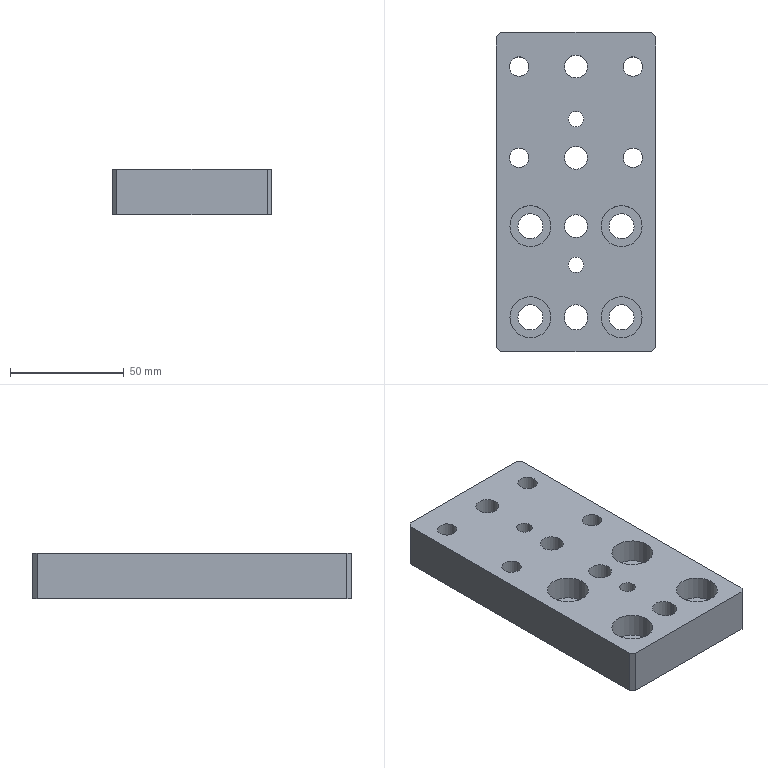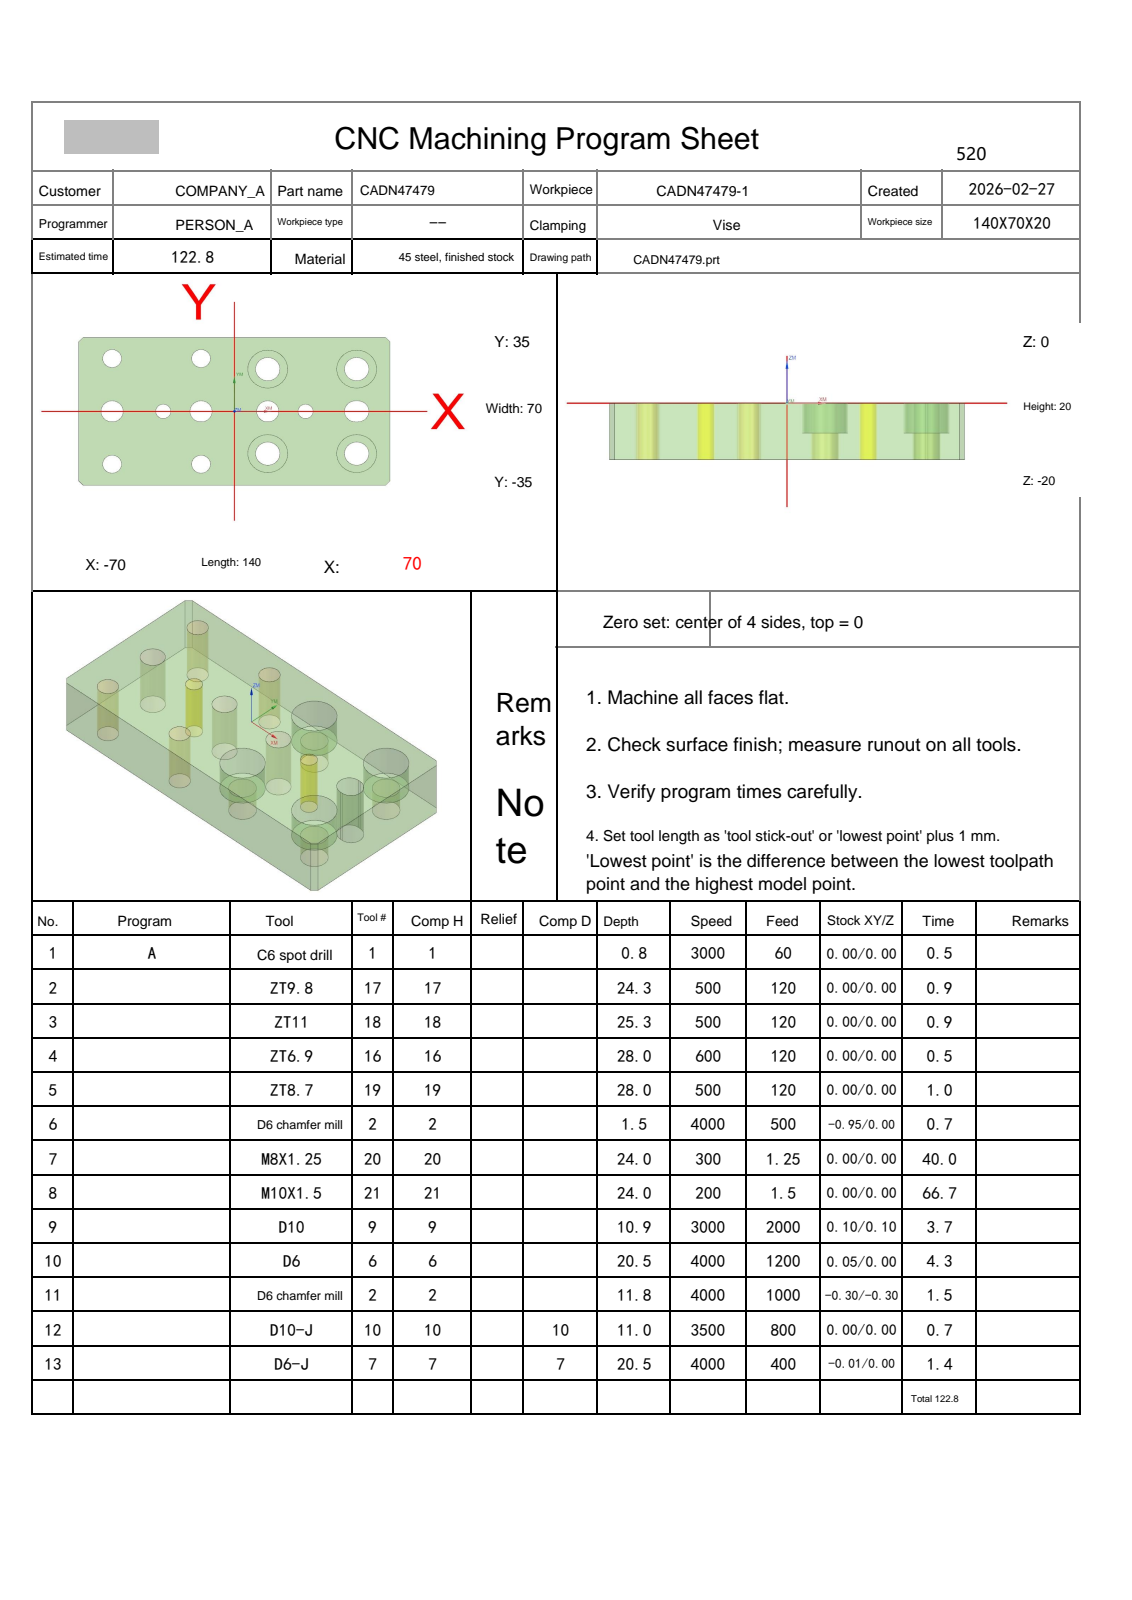NC program | NX | posted by the shop | part box 70 x 140 x 20 mm
Lines 1 to 1647 of 3634, first 1188 of 1645 lines:
%
O0001
(Machine time: 227.62 MIN)
(===Total Tool:12===)
(T1=C6 spot drill   D=6.   R=0.   D-  H01 Z=-0.8  )
(T17=ZT9.8  D=9.8  DR_a=120 D-  H17 Z=-24.33)
(T18=ZT11   D=11.  DR_a=118 D-  H18 Z=-25.3 )
(T16=ZT6.9  D=6.9  DR_a=120 D-  H16 Z=-28.  )
(T19=ZT8.7  D=8.7  DR_a=118 D-  H19 Z=-28.  )
(T2=D6 chamfer mill   D=6.   R=0.   D-  H02 Z=-11.8 )
(T20=M8X1.25 D=6.8  DR_a=180 D-  H20 Z=-24.  )
(T21=M10X1.5 D=8.5  DR_a=180 D-  H21 Z=-24.  )
(T9=D10     D=10.  R=0.   D-  H09 Z=-10.9 )
(T6=D6      D=6.   R=0.   D-  H06 Z=-20.5 )
(T10=D10-J  D=10.  R=0.   D10 H10 Z=-11.  )
(T7=D6-J    D=6.   R=0.   D7  H07 Z=-20.5 )
G80 G90 G17 G49 G40
G91 G28 Z0
M01
N1 T01 M06
(C6 spot drill  D=6. R=0. H=01 ce=0.00 di=0.00)
G00 G90 G54 X55. Y20. M03 S3000
G43 H01 Z30.
M08
G98 G81 X55. Y20. Z-.8 R1. F60.
Y-20.
X32. Y0.0
X15. Y-20.
Y0.0
Y20.
X-15. Y25.
Y0.0
X-32.
X-15. Y-25.
X-55.
Y0.0
Y25.
G80
G00 Z30.
G00 G90 X54.5 Y0.0 M03 S3000
Z30.
G98 G81 X54.5 Y0.0 Z-.8 R1. F60.
G80
G00 Z30.
G91 G28 Z0.0
M05
M09
G91 G28 Z0.0
M01
N2 T17 M06
(ZT9.8 D=9.8 DR_a=120 H=17)
G00 G90 G54 X-55. Y0.0 M03 S500
G43 H17 Z30.
M08
G98 G83 X-55. Y0.0 Z-24.329 R1. F120. Q2.
X-15.
X15.
G80
G00 Z30.
G00 G90 X54.5 Y0.0 M03 S500
Z30.
G98 G83 X54.5 Y0.0 Z-24.329 R1. F120. Q2.
G80
G00 Z30.
G91 G28 Z0.0
M05
M09
G91 G28 Z0.0
M01
N3 T18 M06
(ZT11 D=11. DR_a=118 H=18)
G00 G90 G54 X15. Y-20. M03 S500
G43 H18 Z30.
M08
G98 G83 X15. Y-20. Z-25.305 R1. F120. Q2.
Y20.
X55.
Y-20.
G80
G00 Z30.
G91 G28 Z0.0
M05
M09
G91 G28 Z0.0
M01
N4 T16 M06
(ZT6.9 D=6.9 DR_a=120 H=16)
G00 G90 G54 X-32. Y0.0 M03 S600
G43 H16 Z30.
M08
G98 G83 X-32. Y0.0 Z-28. R1. F120. Q2.
X32.
G80
G00 Z30.
G91 G28 Z0.0
M05
M09
G91 G28 Z0.0
M01
N5 T19 M06
(ZT8.7 D=8.7 DR_a=118 H=19)
G00 G90 G54 X-55. Y-25. M03 S500
G43 H19 Z30.
M08
G98 G83 X-55. Y-25. Z-28. R1. F120. Q2.
X-15.
Y25.
X-55.
G80
G00 Z30.
G91 G28 Z0.0
M05
M09
G91 G28 Z0.0
M01
N6 T02 M06
(D6 chamfer mill  D=6. R=0. H=02 ce=-0.80 di=0.00)
G00 G90 G54 X-33.5 Y-.8 M03 S4000
G43 H02 Z30.
M08
Z-1.
G01 Z-1.5 F500.
Y-1.2
G03 X-32. Y-2.7 I1.5 J0.0
X-29.3 Y0.0 I0.0 J2.7
X-32. Y2.7 I-2.7 J0.0
X-34.7 Y0.0 I0.0 J-2.7
X-32. Y-2.7 I2.7 J0.0
X-30.5 Y-1.2 I0.0 J1.5
G01 Y-.8
Z-1.
G00 Z30.
X30.5
Z-1.
G01 Z-1.5
Y-1.2
G03 X32. Y-2.7 I1.5 J0.0
X34.7 Y0.0 I0.0 J2.7
X32. Y2.7 I-2.7 J0.0
X29.3 Y0.0 I0.0 J-2.7
X32. Y-2.7 I2.7 J0.0
X33.5 Y-1.2 I0.0 J1.5
G01 Y-.8
Z-1.
G00 Z30.
G00 G90 X-57.629 Y24.386 M03 S4000
Z30.
Z-1.
G01 Z-1.5 F500.
X-58. Y24.3
G03 X-55. Y21.3 I3. J0.0
X-51.3 Y25. I0.0 J3.7
X-55. Y28.7 I-3.7 J0.0
X-58.7 Y25. I0.0 J-3.7
X-55. Y21.3 I3.7 J0.0
X-52. Y24.3 I0.0 J3.
G01 X-52.371 Y24.386
Z-1.
G00 Z30.
X-17.629
Z-1.
G01 Z-1.5
X-18. Y24.3
G03 X-15. Y21.3 I3. J0.0
X-11.3 Y25. I0.0 J3.7
X-15. Y28.7 I-3.7 J0.0
X-18.7 Y25. I0.0 J-3.7
X-15. Y21.3 I3.7 J0.0
X-12. Y24.3 I0.0 J3.
G01 X-12.371 Y24.386
Z-1.
G00 Z30.
X-17.629 Y-25.614
Z-1.
G01 Z-1.5
X-18. Y-25.7
G03 X-15. Y-28.7 I3. J0.0
X-11.3 Y-25. I0.0 J3.7
X-15. Y-21.3 I-3.7 J0.0
X-18.7 Y-25. I0.0 J-3.7
X-15. Y-28.7 I3.7 J0.0
X-12. Y-25.7 I0.0 J3.
G01 X-12.371 Y-25.614
Z-1.
G00 Z30.
X-57.629
Z-1.
G01 Z-1.5
X-58. Y-25.7
G03 X-55. Y-28.7 I3. J0.0
X-51.3 Y-25. I0.0 J3.7
X-55. Y-21.3 I-3.7 J0.0
X-58.7 Y-25. I0.0 J-3.7
X-55. Y-28.7 I3.7 J0.0
X-52. Y-25.7 I0.0 J3.
G01 X-52.371 Y-25.614
Z-1.
G00 Z30.
G00 G90 X-58. Y-1.3 M03 S4000
Z30.
Z-.5
G01 Z-1. F500.
G03 X-55. Y-4.3 I3. J0.0
X-50.7 Y0.0 I0.0 J4.3
X-55. Y4.3 I-4.3 J0.0
X-59.3 Y0.0 I0.0 J-4.3
X-55. Y-4.3 I4.3 J0.0
X-52. Y-1.3 I0.0 J3.
G01 Z-.5
G00 Z30.
X-18.
Z-.5
G01 Z-1.
G03 X-15. Y-4.3 I3. J0.0
X-10.7 Y0.0 I0.0 J4.3
X-15. Y4.3 I-4.3 J0.0
X-19.3 Y0.0 I0.0 J-4.3
X-15. Y-4.3 I4.3 J0.0
X-12. Y-1.3 I0.0 J3.
G01 Z-.5
G00 Z30.
X12.
Z-.5
G01 Z-1.
G03 X15. Y-4.3 I3. J0.0
X19.3 Y0.0 I0.0 J4.3
X15. Y4.3 I-4.3 J0.0
X10.7 Y0.0 I0.0 J-4.3
X15. Y-4.3 I4.3 J0.0
X18. Y-1.3 I0.0 J3.
G01 Z-.5
G00 Z30.
G91 G28 Z0.0
M05
M09
G91 G28 Z0.0
M01
N7 T20 M06
(M8X1.25 D=6.8 DR_a=180 H=20)
G00 G90 G54 X-32. Y0.0 M03 S300
G43 H20 Z30.
M08
G95
G98 G84 X-32. Y0.0 Z-24. R1. F1.25 Q3.
X32.
G80
G94
G00 Z30.
G91 G28 Z0.0
M05
M09
G91 G28 Z0.0
M01
N8 T21 M06
(M10X1.5 D=8.5 DR_a=180 H=21)
G00 G90 G54 X-55. Y-25. M03 S200
G43 H21 Z30.
M08
G95
G98 G84 X-55. Y-25. Z-24. R1. F1.5 Q2.
X-15.
Y25.
X-55.
G80
G94
G00 Z30.
G91 G28 Z0.0
M05
M09
G91 G28 Z0.0
M01
N9 T09 M06
(D10  D=10. R=0. H=09 ce=0.10 di=0.10)
G00 G90 G54 X55.636 Y-16.134 M03 S3000
G43 H09 Z30.
M08
Z1.
G01 X54.515 Y-16.1 Z.941 F2000.
X53.275 Y-16.469 Z.873
X52.221 Y-17.221 Z.805
X51.469 Y-18.275 Z.738
X51.1 Y-19.515 Z.67
Y-20.485 Z.619
X51.469 Y-21.725 Z.551
X52.221 Y-22.779 Z.483
X53.275 Y-23.531 Z.415
X54.515 Y-23.9 Z.348
X55.485 Z.297
X56.725 Y-23.531 Z.229
X57.779 Y-22.779 Z.161
X58.531 Y-21.725 Z.093
X58.9 Y-20.485 Z.025
Y-20. Z0.0
G03 X57.321 Y-16.866 Z-.029 I-3.9 J0.0
X55. Y-16.1 Z-.05 I-2.321 J-3.134
X51.1 Y-20. Z-.099 I0.0 J-3.9
X55. Y-23.9 Z-.149 I3.9 J0.0
X58.9 Y-20. Z-.198 I0.0 J3.9
X57.321 Y-16.866 Z-.228 I-3.9 J0.0
X55. Y-16.1 Z-.248 I-2.321 J-3.134
X51.1 Y-20. Z-.297 I0.0 J-3.9
X55. Y-23.9 Z-.347 I3.9 J0.0
X58.9 Y-20. Z-.396 I0.0 J3.9
X57.321 Y-16.866 Z-.426 I-3.9 J0.0
X55. Y-16.1 Z-.446 I-2.321 J-3.134
X51.1 Y-20. Z-.495 I0.0 J-3.9
X55. Y-23.9 Z-.545 I3.9 J0.0
X58.9 Y-20. Z-.594 I0.0 J3.9
X57.321 Y-16.866 Z-.624 I-3.9 J0.0
X55. Y-16.1 Z-.644 I-2.321 J-3.134
X51.1 Y-20. Z-.693 I0.0 J-3.9
X55. Y-23.9 Z-.743 I3.9 J0.0
X58.9 Y-20. Z-.792 I0.0 J3.9
X57.321 Y-16.866 Z-.822 I-3.9 J0.0
X55. Y-16.1 Z-.842 I-2.321 J-3.134
X51.1 Y-20. Z-.892 I0.0 J-3.9
X55. Y-23.9 Z-.941 I3.9 J0.0
X58.9 Y-20. Z-.991 I0.0 J3.9
X57.321 Y-16.866 Z-1.02 I-3.9 J0.0
X55. Y-16.1 Z-1.04 I-2.321 J-3.134
X51.1 Y-20. Z-1.09 I0.0 J-3.9
X55. Y-23.9 Z-1.139 I3.9 J0.0
X58.9 Y-20. Z-1.189 I0.0 J3.9
X57.321 Y-16.866 Z-1.218 I-3.9 J0.0
X55. Y-16.1 Z-1.238 I-2.321 J-3.134
X51.1 Y-20. Z-1.288 I0.0 J-3.9
X55. Y-23.9 Z-1.337 I3.9 J0.0
X58.9 Y-20. Z-1.387 I0.0 J3.9
X57.321 Y-16.866 Z-1.416 I-3.9 J0.0
X55. Y-16.1 Z-1.436 I-2.321 J-3.134
X51.1 Y-20. Z-1.486 I0.0 J-3.9
X55. Y-23.9 Z-1.535 I3.9 J0.0
X58.9 Y-20. Z-1.585 I0.0 J3.9
X57.321 Y-16.866 Z-1.614 I-3.9 J0.0
X55. Y-16.1 Z-1.634 I-2.321 J-3.134
X51.1 Y-20. Z-1.684 I0.0 J-3.9
X55. Y-23.9 Z-1.733 I3.9 J0.0
X58.9 Y-20. Z-1.783 I0.0 J3.9
X57.321 Y-16.866 Z-1.812 I-3.9 J0.0
X55. Y-16.1 Z-1.833 I-2.321 J-3.134
X51.1 Y-20. Z-1.882 I0.0 J-3.9
X55. Y-23.9 Z-1.932 I3.9 J0.0
X58.9 Y-20. Z-1.981 I0.0 J3.9
X57.321 Y-16.866 Z-2.011 I-3.9 J0.0
X55. Y-16.1 Z-2.031 I-2.321 J-3.134
X51.1 Y-20. Z-2.08 I0.0 J-3.9
X55. Y-23.9 Z-2.13 I3.9 J0.0
X58.9 Y-20. Z-2.179 I0.0 J3.9
X57.321 Y-16.866 Z-2.209 I-3.9 J0.0
X55. Y-16.1 Z-2.229 I-2.321 J-3.134
X51.1 Y-20. Z-2.278 I0.0 J-3.9
X55. Y-23.9 Z-2.328 I3.9 J0.0
X58.9 Y-20. Z-2.377 I0.0 J3.9
X57.321 Y-16.866 Z-2.407 I-3.9 J0.0
X55. Y-16.1 Z-2.427 I-2.321 J-3.134
X51.1 Y-20. Z-2.476 I0.0 J-3.9
X55. Y-23.9 Z-2.526 I3.9 J0.0
X58.9 Y-20. Z-2.575 I0.0 J3.9
X57.321 Y-16.866 Z-2.605 I-3.9 J0.0
X55. Y-16.1 Z-2.625 I-2.321 J-3.134
X51.1 Y-20. Z-2.675 I0.0 J-3.9
X55. Y-23.9 Z-2.724 I3.9 J0.0
X58.9 Y-20. Z-2.774 I0.0 J3.9
X57.321 Y-16.866 Z-2.803 I-3.9 J0.0
X55. Y-16.1 Z-2.823 I-2.321 J-3.134
X51.1 Y-20. Z-2.873 I0.0 J-3.9
X55. Y-23.9 Z-2.922 I3.9 J0.0
X58.9 Y-20. Z-2.972 I0.0 J3.9
X57.321 Y-16.866 Z-3.001 I-3.9 J0.0
X55. Y-16.1 Z-3.021 I-2.321 J-3.134
X51.1 Y-20. Z-3.071 I0.0 J-3.9
X55. Y-23.9 Z-3.12 I3.9 J0.0
X58.9 Y-20. Z-3.17 I0.0 J3.9
X57.321 Y-16.866 Z-3.199 I-3.9 J0.0
X55. Y-16.1 Z-3.219 I-2.321 J-3.134
X51.1 Y-20. Z-3.269 I0.0 J-3.9
X55. Y-23.9 Z-3.318 I3.9 J0.0
X58.9 Y-20. Z-3.368 I0.0 J3.9
X57.321 Y-16.866 Z-3.397 I-3.9 J0.0
X55. Y-16.1 Z-3.417 I-2.321 J-3.134
X51.1 Y-20. Z-3.467 I0.0 J-3.9
X55. Y-23.9 Z-3.517 I3.9 J0.0
X58.9 Y-20. Z-3.566 I0.0 J3.9
X57.321 Y-16.866 Z-3.595 I-3.9 J0.0
X55. Y-16.1 Z-3.616 I-2.321 J-3.134
X51.1 Y-20. Z-3.665 I0.0 J-3.9
X55. Y-23.9 Z-3.715 I3.9 J0.0
X58.9 Y-20. Z-3.764 I0.0 J3.9
X57.321 Y-16.866 Z-3.794 I-3.9 J0.0
X55. Y-16.1 Z-3.814 I-2.321 J-3.134
X51.1 Y-20. Z-3.863 I0.0 J-3.9
X55. Y-23.9 Z-3.913 I3.9 J0.0
X58.9 Y-20. Z-3.962 I0.0 J3.9
X57.321 Y-16.866 Z-3.992 I-3.9 J0.0
X55. Y-16.1 Z-4.012 I-2.321 J-3.134
X51.1 Y-20. Z-4.061 I0.0 J-3.9
X55. Y-23.9 Z-4.111 I3.9 J0.0
X58.9 Y-20. Z-4.16 I0.0 J3.9
X57.321 Y-16.866 Z-4.19 I-3.9 J0.0
X55. Y-16.1 Z-4.21 I-2.321 J-3.134
X51.1 Y-20. Z-4.259 I0.0 J-3.9
X55. Y-23.9 Z-4.309 I3.9 J0.0
X58.9 Y-20. Z-4.358 I0.0 J3.9
X57.321 Y-16.866 Z-4.388 I-3.9 J0.0
X55. Y-16.1 Z-4.408 I-2.321 J-3.134
X51.1 Y-20. Z-4.458 I0.0 J-3.9
X55. Y-23.9 Z-4.507 I3.9 J0.0
X58.9 Y-20. Z-4.557 I0.0 J3.9
X57.321 Y-16.866 Z-4.586 I-3.9 J0.0
X55. Y-16.1 Z-4.606 I-2.321 J-3.134
X51.1 Y-20. Z-4.656 I0.0 J-3.9
X55. Y-23.9 Z-4.705 I3.9 J0.0
X58.9 Y-20. Z-4.755 I0.0 J3.9
X57.321 Y-16.866 Z-4.784 I-3.9 J0.0
X55. Y-16.1 Z-4.804 I-2.321 J-3.134
X51.1 Y-20. Z-4.854 I0.0 J-3.9
X55. Y-23.9 Z-4.903 I3.9 J0.0
X58.9 Y-20. Z-4.953 I0.0 J3.9
X57.321 Y-16.866 Z-4.982 I-3.9 J0.0
X55. Y-16.1 Z-5.002 I-2.321 J-3.134
X51.1 Y-20. Z-5.052 I0.0 J-3.9
X55. Y-23.9 Z-5.101 I3.9 J0.0
X58.9 Y-20. Z-5.151 I0.0 J3.9
X57.321 Y-16.866 Z-5.18 I-3.9 J0.0
X55. Y-16.1 Z-5.2 I-2.321 J-3.134
X51.1 Y-20. Z-5.25 I0.0 J-3.9
X55. Y-23.9 Z-5.3 I3.9 J0.0
X58.9 Y-20. Z-5.349 I0.0 J3.9
X57.321 Y-16.866 Z-5.378 I-3.9 J0.0
X55. Y-16.1 Z-5.399 I-2.321 J-3.134
X51.1 Y-20. Z-5.448 I0.0 J-3.9
X55. Y-23.9 Z-5.498 I3.9 J0.0
X58.9 Y-20. Z-5.547 I0.0 J3.9
X57.321 Y-16.866 Z-5.577 I-3.9 J0.0
X55. Y-16.1 Z-5.597 I-2.321 J-3.134
X51.1 Y-20. Z-5.646 I0.0 J-3.9
X55. Y-23.9 Z-5.696 I3.9 J0.0
X58.9 Y-20. Z-5.745 I0.0 J3.9
X57.321 Y-16.866 Z-5.775 I-3.9 J0.0
X55. Y-16.1 Z-5.795 I-2.321 J-3.134
X51.1 Y-20. Z-5.844 I0.0 J-3.9
X55. Y-23.9 Z-5.894 I3.9 J0.0
X58.9 Y-20. Z-5.943 I0.0 J3.9
X57.321 Y-16.866 Z-5.973 I-3.9 J0.0
X55. Y-16.1 Z-5.993 I-2.321 J-3.134
X51.1 Y-20. Z-6.042 I0.0 J-3.9
X55. Y-23.9 Z-6.092 I3.9 J0.0
X58.9 Y-20. Z-6.142 I0.0 J3.9
X57.321 Y-16.866 Z-6.171 I-3.9 J0.0
X55. Y-16.1 Z-6.191 I-2.321 J-3.134
X51.1 Y-20. Z-6.241 I0.0 J-3.9
X55. Y-23.9 Z-6.29 I3.9 J0.0
X58.9 Y-20. Z-6.34 I0.0 J3.9
X57.321 Y-16.866 Z-6.369 I-3.9 J0.0
X55. Y-16.1 Z-6.389 I-2.321 J-3.134
X51.1 Y-20. Z-6.439 I0.0 J-3.9
X55. Y-23.9 Z-6.488 I3.9 J0.0
X58.9 Y-20. Z-6.538 I0.0 J3.9
X57.321 Y-16.866 Z-6.567 I-3.9 J0.0
X55. Y-16.1 Z-6.587 I-2.321 J-3.134
X51.1 Y-20. Z-6.637 I0.0 J-3.9
X55. Y-23.9 Z-6.686 I3.9 J0.0
X58.9 Y-20. Z-6.736 I0.0 J3.9
X57.321 Y-16.866 Z-6.765 I-3.9 J0.0
X55. Y-16.1 Z-6.785 I-2.321 J-3.134
X51.1 Y-20. Z-6.835 I0.0 J-3.9
X55. Y-23.9 Z-6.884 I3.9 J0.0
X58.9 Y-20. Z-6.934 I0.0 J3.9
X57.321 Y-16.866 Z-6.963 I-3.9 J0.0
X55. Y-16.1 Z-6.983 I-2.321 J-3.134
X51.1 Y-20. Z-7.033 I0.0 J-3.9
X55. Y-23.9 Z-7.083 I3.9 J0.0
X58.9 Y-20. Z-7.132 I0.0 J3.9
X57.321 Y-16.866 Z-7.162 I-3.9 J0.0
X55. Y-16.1 Z-7.182 I-2.321 J-3.134
X51.1 Y-20. Z-7.231 I0.0 J-3.9
X55. Y-23.9 Z-7.281 I3.9 J0.0
X58.9 Y-20. Z-7.33 I0.0 J3.9
X57.321 Y-16.866 Z-7.36 I-3.9 J0.0
X55. Y-16.1 Z-7.38 I-2.321 J-3.134
X51.1 Y-20. Z-7.429 I0.0 J-3.9
X55. Y-23.9 Z-7.479 I3.9 J0.0
X58.9 Y-20. Z-7.528 I0.0 J3.9
X57.321 Y-16.866 Z-7.558 I-3.9 J0.0
X55. Y-16.1 Z-7.578 I-2.321 J-3.134
X51.1 Y-20. Z-7.627 I0.0 J-3.9
X55. Y-23.9 Z-7.677 I3.9 J0.0
X58.9 Y-20. Z-7.726 I0.0 J3.9
X57.321 Y-16.866 Z-7.756 I-3.9 J0.0
X55. Y-16.1 Z-7.776 I-2.321 J-3.134
X51.1 Y-20. Z-7.825 I0.0 J-3.9
X55. Y-23.9 Z-7.875 I3.9 J0.0
X58.9 Y-20. Z-7.925 I0.0 J3.9
X57.321 Y-16.866 Z-7.954 I-3.9 J0.0
X55. Y-16.1 Z-7.974 I-2.321 J-3.134
X51.1 Y-20. Z-8.024 I0.0 J-3.9
X55. Y-23.9 Z-8.073 I3.9 J0.0
X58.9 Y-20. Z-8.123 I0.0 J3.9
X57.321 Y-16.866 Z-8.152 I-3.9 J0.0
X55. Y-16.1 Z-8.172 I-2.321 J-3.134
X51.1 Y-20. Z-8.222 I0.0 J-3.9
X55. Y-23.9 Z-8.271 I3.9 J0.0
X58.9 Y-20. Z-8.321 I0.0 J3.9
X57.321 Y-16.866 Z-8.35 I-3.9 J0.0
X55. Y-16.1 Z-8.37 I-2.321 J-3.134
X51.1 Y-20. Z-8.42 I0.0 J-3.9
X55. Y-23.9 Z-8.469 I3.9 J0.0
X58.9 Y-20. Z-8.519 I0.0 J3.9
X57.321 Y-16.866 Z-8.548 I-3.9 J0.0
X55. Y-16.1 Z-8.568 I-2.321 J-3.134
X51.1 Y-20. Z-8.618 I0.0 J-3.9
X55. Y-23.9 Z-8.667 I3.9 J0.0
X58.9 Y-20. Z-8.717 I0.0 J3.9
X57.321 Y-16.866 Z-8.746 I-3.9 J0.0
X55. Y-16.1 Z-8.767 I-2.321 J-3.134
X51.1 Y-20. Z-8.816 I0.0 J-3.9
X55. Y-23.9 Z-8.866 I3.9 J0.0
X58.9 Y-20. Z-8.915 I0.0 J3.9
X57.321 Y-16.866 Z-8.945 I-3.9 J0.0
X55. Y-16.1 Z-8.965 I-2.321 J-3.134
X51.1 Y-20. Z-9.014 I0.0 J-3.9
X55. Y-23.9 Z-9.064 I3.9 J0.0
X58.9 Y-20. Z-9.113 I0.0 J3.9
X57.321 Y-16.866 Z-9.143 I-3.9 J0.0
X55. Y-16.1 Z-9.163 I-2.321 J-3.134
X51.1 Y-20. Z-9.212 I0.0 J-3.9
X55. Y-23.9 Z-9.262 I3.9 J0.0
X58.9 Y-20. Z-9.311 I0.0 J3.9
X57.321 Y-16.866 Z-9.341 I-3.9 J0.0
X55. Y-16.1 Z-9.361 I-2.321 J-3.134
X51.1 Y-20. Z-9.41 I0.0 J-3.9
X55. Y-23.9 Z-9.46 I3.9 J0.0
X58.9 Y-20. Z-9.509 I0.0 J3.9
X57.321 Y-16.866 Z-9.539 I-3.9 J0.0
X55. Y-16.1 Z-9.559 I-2.321 J-3.134
X51.1 Y-20. Z-9.608 I0.0 J-3.9
X55. Y-23.9 Z-9.658 I3.9 J0.0
X58.9 Y-20. Z-9.708 I0.0 J3.9
X57.321 Y-16.866 Z-9.737 I-3.9 J0.0
X55. Y-16.1 Z-9.757 I-2.321 J-3.134
X51.1 Y-20. Z-9.807 I0.0 J-3.9
X55. Y-23.9 Z-9.856 I3.9 J0.0
X58.9 Y-20. Z-9.906 I0.0 J3.9
X57.321 Y-16.866 Z-9.935 I-3.9 J0.0
X55. Y-16.1 Z-9.955 I-2.321 J-3.134
X51.1 Y-20. Z-10.005 I0.0 J-3.9
X55. Y-23.9 Z-10.054 I3.9 J0.0
X58.9 Y-20. Z-10.104 I0.0 J3.9
X57.321 Y-16.866 Z-10.133 I-3.9 J0.0
X55. Y-16.1 Z-10.153 I-2.321 J-3.134
X51.1 Y-20. Z-10.203 I0.0 J-3.9
X55. Y-23.9 Z-10.252 I3.9 J0.0
X58.9 Y-20. Z-10.302 I0.0 J3.9
X57.321 Y-16.866 Z-10.331 I-3.9 J0.0
X55. Y-16.1 Z-10.351 I-2.321 J-3.134
X51.1 Y-20. Z-10.401 I0.0 J-3.9
X55. Y-23.9 Z-10.45 I3.9 J0.0
X58.9 Y-20. Z-10.5 I0.0 J3.9
X55. Y-16.1 I-3.9 J0.0
X51.1 Y-20. I0.0 J-3.9
X55. Y-23.9 I3.9 J0.0
X58.9 Y-20. I0.0 J3.9
X58.88 Y-19.601 I-3.9 J0.0
G01 Z-9.5
G00 Z30.
X18.856 Y-20.634
Z1.
G01 X18.9 Y-20.485 Z.992
Y-19.515 Z.941
X18.531 Y-18.275 Z.873
X17.779 Y-17.221 Z.805
X16.725 Y-16.469 Z.738
X15.485 Y-16.1 Z.67
X14.515 Z.619
X13.275 Y-16.469 Z.551
X12.221 Y-17.221 Z.483
X11.469 Y-18.275 Z.415
X11.1 Y-19.515 Z.348
Y-20.485 Z.297
X11.469 Y-21.725 Z.229
X12.221 Y-22.779 Z.161
X13.275 Y-23.531 Z.093
X14.515 Y-23.9 Z.025
X15. Z0.0
G03 X18.9 Y-20. Z-.05 I0.0 J3.9
X15. Y-16.1 Z-.099 I-3.9 J0.0
X11.1 Y-20. Z-.149 I0.0 J-3.9
X15. Y-23.9 Z-.198 I3.9 J0.0
X18.9 Y-20. Z-.248 I0.0 J3.9
X15. Y-16.1 Z-.297 I-3.9 J0.0
X11.1 Y-20. Z-.347 I0.0 J-3.9
X15. Y-23.9 Z-.396 I3.9 J0.0
X18.9 Y-20. Z-.446 I0.0 J3.9
X15. Y-16.1 Z-.495 I-3.9 J0.0
X11.1 Y-20. Z-.545 I0.0 J-3.9
X15. Y-23.9 Z-.594 I3.9 J0.0
X18.9 Y-20. Z-.644 I0.0 J3.9
X15. Y-16.1 Z-.693 I-3.9 J0.0
X11.1 Y-20. Z-.743 I0.0 J-3.9
X15. Y-23.9 Z-.792 I3.9 J0.0
X18.9 Y-20. Z-.842 I0.0 J3.9
X15. Y-16.1 Z-.892 I-3.9 J0.0
X11.1 Y-20. Z-.941 I0.0 J-3.9
X15. Y-23.9 Z-.991 I3.9 J0.0
X18.9 Y-20. Z-1.04 I0.0 J3.9
X15. Y-16.1 Z-1.09 I-3.9 J0.0
X11.1 Y-20. Z-1.139 I0.0 J-3.9
X15. Y-23.9 Z-1.189 I3.9 J0.0
X18.9 Y-20. Z-1.238 I0.0 J3.9
X15. Y-16.1 Z-1.288 I-3.9 J0.0
X11.1 Y-20. Z-1.337 I0.0 J-3.9
X15. Y-23.9 Z-1.387 I3.9 J0.0
X18.9 Y-20. Z-1.436 I0.0 J3.9
X15. Y-16.1 Z-1.486 I-3.9 J0.0
X11.1 Y-20. Z-1.535 I0.0 J-3.9
X15. Y-23.9 Z-1.585 I3.9 J0.0
X18.9 Y-20. Z-1.634 I0.0 J3.9
X15. Y-16.1 Z-1.684 I-3.9 J0.0
X11.1 Y-20. Z-1.733 I0.0 J-3.9
X15. Y-23.9 Z-1.783 I3.9 J0.0
X18.9 Y-20. Z-1.833 I0.0 J3.9
X15. Y-16.1 Z-1.882 I-3.9 J0.0
X11.1 Y-20. Z-1.932 I0.0 J-3.9
X15. Y-23.9 Z-1.981 I3.9 J0.0
X18.9 Y-20. Z-2.031 I0.0 J3.9
X15. Y-16.1 Z-2.08 I-3.9 J0.0
X11.1 Y-20. Z-2.13 I0.0 J-3.9
X15. Y-23.9 Z-2.179 I3.9 J0.0
X18.9 Y-20. Z-2.229 I0.0 J3.9
X15. Y-16.1 Z-2.278 I-3.9 J0.0
X11.1 Y-20. Z-2.328 I0.0 J-3.9
X15. Y-23.9 Z-2.377 I3.9 J0.0
X18.9 Y-20. Z-2.427 I0.0 J3.9
X15. Y-16.1 Z-2.476 I-3.9 J0.0
X11.1 Y-20. Z-2.526 I0.0 J-3.9
X15. Y-23.9 Z-2.575 I3.9 J0.0
X18.9 Y-20. Z-2.625 I0.0 J3.9
X15. Y-16.1 Z-2.675 I-3.9 J0.0
X11.1 Y-20. Z-2.724 I0.0 J-3.9
X15. Y-23.9 Z-2.774 I3.9 J0.0
X18.9 Y-20. Z-2.823 I0.0 J3.9
X15. Y-16.1 Z-2.873 I-3.9 J0.0
X11.1 Y-20. Z-2.922 I0.0 J-3.9
X15. Y-23.9 Z-2.972 I3.9 J0.0
X18.9 Y-20. Z-3.021 I0.0 J3.9
X15. Y-16.1 Z-3.071 I-3.9 J0.0
X11.1 Y-20. Z-3.12 I0.0 J-3.9
X15. Y-23.9 Z-3.17 I3.9 J0.0
X18.9 Y-20. Z-3.219 I0.0 J3.9
X15. Y-16.1 Z-3.269 I-3.9 J0.0
X11.1 Y-20. Z-3.318 I0.0 J-3.9
X15. Y-23.9 Z-3.368 I3.9 J0.0
X18.9 Y-20. Z-3.417 I0.0 J3.9
X15. Y-16.1 Z-3.467 I-3.9 J0.0
X11.1 Y-20. Z-3.517 I0.0 J-3.9
X15. Y-23.9 Z-3.566 I3.9 J0.0
X18.9 Y-20. Z-3.616 I0.0 J3.9
X15. Y-16.1 Z-3.665 I-3.9 J0.0
X11.1 Y-20. Z-3.715 I0.0 J-3.9
X15. Y-23.9 Z-3.764 I3.9 J0.0
X18.9 Y-20. Z-3.814 I0.0 J3.9
X15. Y-16.1 Z-3.863 I-3.9 J0.0
X11.1 Y-20. Z-3.913 I0.0 J-3.9
X15. Y-23.9 Z-3.962 I3.9 J0.0
X18.9 Y-20. Z-4.012 I0.0 J3.9
X15. Y-16.1 Z-4.061 I-3.9 J0.0
X11.1 Y-20. Z-4.111 I0.0 J-3.9
X15. Y-23.9 Z-4.16 I3.9 J0.0
X18.9 Y-20. Z-4.21 I0.0 J3.9
X15. Y-16.1 Z-4.259 I-3.9 J0.0
X11.1 Y-20. Z-4.309 I0.0 J-3.9
X15. Y-23.9 Z-4.358 I3.9 J0.0
X18.9 Y-20. Z-4.408 I0.0 J3.9
X15. Y-16.1 Z-4.458 I-3.9 J0.0
X11.1 Y-20. Z-4.507 I0.0 J-3.9
X15. Y-23.9 Z-4.557 I3.9 J0.0
X18.9 Y-20. Z-4.606 I0.0 J3.9
X15. Y-16.1 Z-4.656 I-3.9 J0.0
X11.1 Y-20. Z-4.705 I0.0 J-3.9
X15. Y-23.9 Z-4.755 I3.9 J0.0
X18.9 Y-20. Z-4.804 I0.0 J3.9
X15. Y-16.1 Z-4.854 I-3.9 J0.0
X11.1 Y-20. Z-4.903 I0.0 J-3.9
X15. Y-23.9 Z-4.953 I3.9 J0.0
X18.9 Y-20. Z-5.002 I0.0 J3.9
X15. Y-16.1 Z-5.052 I-3.9 J0.0
X11.1 Y-20. Z-5.101 I0.0 J-3.9
X15. Y-23.9 Z-5.151 I3.9 J0.0
X18.9 Y-20. Z-5.2 I0.0 J3.9
X15. Y-16.1 Z-5.25 I-3.9 J0.0
X11.1 Y-20. Z-5.3 I0.0 J-3.9
X15. Y-23.9 Z-5.349 I3.9 J0.0
X18.9 Y-20. Z-5.399 I0.0 J3.9
X15. Y-16.1 Z-5.448 I-3.9 J0.0
X11.1 Y-20. Z-5.498 I0.0 J-3.9
X15. Y-23.9 Z-5.547 I3.9 J0.0
X18.9 Y-20. Z-5.597 I0.0 J3.9
X15. Y-16.1 Z-5.646 I-3.9 J0.0
X11.1 Y-20. Z-5.696 I0.0 J-3.9
X15. Y-23.9 Z-5.745 I3.9 J0.0
X18.9 Y-20. Z-5.795 I0.0 J3.9
X15. Y-16.1 Z-5.844 I-3.9 J0.0
X11.1 Y-20. Z-5.894 I0.0 J-3.9
X15. Y-23.9 Z-5.943 I3.9 J0.0
X18.9 Y-20. Z-5.993 I0.0 J3.9
X15. Y-16.1 Z-6.042 I-3.9 J0.0
X11.1 Y-20. Z-6.092 I0.0 J-3.9
X15. Y-23.9 Z-6.142 I3.9 J0.0
X18.9 Y-20. Z-6.191 I0.0 J3.9
X15. Y-16.1 Z-6.241 I-3.9 J0.0
X11.1 Y-20. Z-6.29 I0.0 J-3.9
X15. Y-23.9 Z-6.34 I3.9 J0.0
X18.9 Y-20. Z-6.389 I0.0 J3.9
X15. Y-16.1 Z-6.439 I-3.9 J0.0
X11.1 Y-20. Z-6.488 I0.0 J-3.9
X15. Y-23.9 Z-6.538 I3.9 J0.0
X18.9 Y-20. Z-6.587 I0.0 J3.9
X15. Y-16.1 Z-6.637 I-3.9 J0.0
X11.1 Y-20. Z-6.686 I0.0 J-3.9
X15. Y-23.9 Z-6.736 I3.9 J0.0
X18.9 Y-20. Z-6.785 I0.0 J3.9
X15. Y-16.1 Z-6.835 I-3.9 J0.0
X11.1 Y-20. Z-6.884 I0.0 J-3.9
X15. Y-23.9 Z-6.934 I3.9 J0.0
X18.9 Y-20. Z-6.983 I0.0 J3.9
X15. Y-16.1 Z-7.033 I-3.9 J0.0
X11.1 Y-20. Z-7.083 I0.0 J-3.9
X15. Y-23.9 Z-7.132 I3.9 J0.0
X18.9 Y-20. Z-7.182 I0.0 J3.9
X15. Y-16.1 Z-7.231 I-3.9 J0.0
X11.1 Y-20. Z-7.281 I0.0 J-3.9
X15. Y-23.9 Z-7.33 I3.9 J0.0
X18.9 Y-20. Z-7.38 I0.0 J3.9
X15. Y-16.1 Z-7.429 I-3.9 J0.0
X11.1 Y-20. Z-7.479 I0.0 J-3.9
X15. Y-23.9 Z-7.528 I3.9 J0.0
X18.9 Y-20. Z-7.578 I0.0 J3.9
X15. Y-16.1 Z-7.627 I-3.9 J0.0
X11.1 Y-20. Z-7.677 I0.0 J-3.9
X15. Y-23.9 Z-7.726 I3.9 J0.0
X18.9 Y-20. Z-7.776 I0.0 J3.9
X15. Y-16.1 Z-7.825 I-3.9 J0.0
X11.1 Y-20. Z-7.875 I0.0 J-3.9
X15. Y-23.9 Z-7.925 I3.9 J0.0
X18.9 Y-20. Z-7.974 I0.0 J3.9
X15. Y-16.1 Z-8.024 I-3.9 J0.0
X11.1 Y-20. Z-8.073 I0.0 J-3.9
X15. Y-23.9 Z-8.123 I3.9 J0.0
X18.9 Y-20. Z-8.172 I0.0 J3.9
X15. Y-16.1 Z-8.222 I-3.9 J0.0
X11.1 Y-20. Z-8.271 I0.0 J-3.9
X15. Y-23.9 Z-8.321 I3.9 J0.0
X18.9 Y-20. Z-8.37 I0.0 J3.9
X15. Y-16.1 Z-8.42 I-3.9 J0.0
X11.1 Y-20. Z-8.469 I0.0 J-3.9
X15. Y-23.9 Z-8.519 I3.9 J0.0
X18.9 Y-20. Z-8.568 I0.0 J3.9
X15. Y-16.1 Z-8.618 I-3.9 J0.0
X11.1 Y-20. Z-8.667 I0.0 J-3.9
X15. Y-23.9 Z-8.717 I3.9 J0.0
X18.9 Y-20. Z-8.767 I0.0 J3.9
X15. Y-16.1 Z-8.816 I-3.9 J0.0
X11.1 Y-20. Z-8.866 I0.0 J-3.9
X15. Y-23.9 Z-8.915 I3.9 J0.0
X18.9 Y-20. Z-8.965 I0.0 J3.9
X15. Y-16.1 Z-9.014 I-3.9 J0.0
X11.1 Y-20. Z-9.064 I0.0 J-3.9
X15. Y-23.9 Z-9.113 I3.9 J0.0
X18.9 Y-20. Z-9.163 I0.0 J3.9
X15. Y-16.1 Z-9.212 I-3.9 J0.0
X11.1 Y-20. Z-9.262 I0.0 J-3.9
X15. Y-23.9 Z-9.311 I3.9 J0.0
X18.9 Y-20. Z-9.361 I0.0 J3.9
X15. Y-16.1 Z-9.41 I-3.9 J0.0
X11.1 Y-20. Z-9.46 I0.0 J-3.9
X15. Y-23.9 Z-9.509 I3.9 J0.0
X18.9 Y-20. Z-9.559 I0.0 J3.9
X15. Y-16.1 Z-9.608 I-3.9 J0.0
X11.1 Y-20. Z-9.658 I0.0 J-3.9
X15. Y-23.9 Z-9.708 I3.9 J0.0
X18.9 Y-20. Z-9.757 I0.0 J3.9
X15. Y-16.1 Z-9.807 I-3.9 J0.0
X11.1 Y-20. Z-9.856 I0.0 J-3.9
X15. Y-23.9 Z-9.906 I3.9 J0.0
X18.9 Y-20. Z-9.955 I0.0 J3.9
X15. Y-16.1 Z-10.005 I-3.9 J0.0
X11.1 Y-20. Z-10.054 I0.0 J-3.9
X15. Y-23.9 Z-10.104 I3.9 J0.0
X18.9 Y-20. Z-10.153 I0.0 J3.9
X15. Y-16.1 Z-10.203 I-3.9 J0.0
X11.1 Y-20. Z-10.252 I0.0 J-3.9
X15. Y-23.9 Z-10.302 I3.9 J0.0
X18.9 Y-20. Z-10.351 I0.0 J3.9
X15. Y-16.1 Z-10.401 I-3.9 J0.0
X11.1 Y-20. Z-10.45 I0.0 J-3.9
X15. Y-23.9 Z-10.5 I3.9 J0.0
X18.9 Y-20. I0.0 J3.9
X15. Y-16.1 I-3.9 J0.0
X11.1 Y-20. I0.0 J-3.9
X15. Y-23.9 I3.9 J0.0
X15.399 Y-23.88 I0.0 J3.9
G01 Z-9.5
G00 Z30.
X11.144 Y20.634
Z1.
G01 X11.1 Y20.485 Z.992
Y19.515 Z.941
X11.469 Y18.275 Z.873
X12.221 Y17.221 Z.805
X13.275 Y16.469 Z.738
X14.515 Y16.1 Z.67
X15.485 Z.619
X16.725 Y16.469 Z.551
X17.779 Y17.221 Z.483
X18.531 Y18.275 Z.415
X18.9 Y19.515 Z.348
Y20.485 Z.297
X18.531 Y21.725 Z.229
X17.779 Y22.779 Z.161
X16.725 Y23.531 Z.093
X15.485 Y23.9 Z.025
X15. Z0.0
G03 X11.1 Y20. Z-.05 I0.0 J-3.9
X15. Y16.1 Z-.099 I3.9 J0.0
X18.9 Y20. Z-.149 I0.0 J3.9
X15. Y23.9 Z-.198 I-3.9 J0.0
X11.1 Y20. Z-.248 I0.0 J-3.9
X15. Y16.1 Z-.297 I3.9 J0.0
X18.9 Y20. Z-.347 I0.0 J3.9
X15. Y23.9 Z-.396 I-3.9 J0.0
X11.1 Y20. Z-.446 I0.0 J-3.9
X15. Y16.1 Z-.495 I3.9 J0.0
X18.9 Y20. Z-.545 I0.0 J3.9
X15. Y23.9 Z-.594 I-3.9 J0.0
X11.1 Y20. Z-.644 I0.0 J-3.9
X15. Y16.1 Z-.693 I3.9 J0.0
X18.9 Y20. Z-.743 I0.0 J3.9
X15. Y23.9 Z-.792 I-3.9 J0.0
X11.1 Y20. Z-.842 I0.0 J-3.9
X15. Y16.1 Z-.892 I3.9 J0.0
X18.9 Y20. Z-.941 I0.0 J3.9
X15. Y23.9 Z-.991 I-3.9 J0.0
X11.1 Y20. Z-1.04 I0.0 J-3.9
X15. Y16.1 Z-1.09 I3.9 J0.0
X18.9 Y20. Z-1.139 I0.0 J3.9
X15. Y23.9 Z-1.189 I-3.9 J0.0
X11.1 Y20. Z-1.238 I0.0 J-3.9
X15. Y16.1 Z-1.288 I3.9 J0.0
X18.9 Y20. Z-1.337 I0.0 J3.9
X15. Y23.9 Z-1.387 I-3.9 J0.0
X11.1 Y20. Z-1.436 I0.0 J-3.9
X15. Y16.1 Z-1.486 I3.9 J0.0
X18.9 Y20. Z-1.535 I0.0 J3.9
X15. Y23.9 Z-1.585 I-3.9 J0.0
X11.1 Y20. Z-1.634 I0.0 J-3.9
X15. Y16.1 Z-1.684 I3.9 J0.0
X18.9 Y20. Z-1.733 I0.0 J3.9
X15. Y23.9 Z-1.783 I-3.9 J0.0
X11.1 Y20. Z-1.833 I0.0 J-3.9
X15. Y16.1 Z-1.882 I3.9 J0.0
X18.9 Y20. Z-1.932 I0.0 J3.9
X15. Y23.9 Z-1.981 I-3.9 J0.0
X11.1 Y20. Z-2.031 I0.0 J-3.9
X15. Y16.1 Z-2.08 I3.9 J0.0
X18.9 Y20. Z-2.13 I0.0 J3.9
X15. Y23.9 Z-2.179 I-3.9 J0.0
X11.1 Y20. Z-2.229 I0.0 J-3.9
X15. Y16.1 Z-2.278 I3.9 J0.0
X18.9 Y20. Z-2.328 I0.0 J3.9
X15. Y23.9 Z-2.377 I-3.9 J0.0
X11.1 Y20. Z-2.427 I0.0 J-3.9
X15. Y16.1 Z-2.476 I3.9 J0.0
X18.9 Y20. Z-2.526 I0.0 J3.9
X15. Y23.9 Z-2.575 I-3.9 J0.0
X11.1 Y20. Z-2.625 I0.0 J-3.9
X15. Y16.1 Z-2.675 I3.9 J0.0
X18.9 Y20. Z-2.724 I0.0 J3.9
X15. Y23.9 Z-2.774 I-3.9 J0.0
X11.1 Y20. Z-2.823 I0.0 J-3.9
X15. Y16.1 Z-2.873 I3.9 J0.0
X18.9 Y20. Z-2.922 I0.0 J3.9
X15. Y23.9 Z-2.972 I-3.9 J0.0
X11.1 Y20. Z-3.021 I0.0 J-3.9
X15. Y16.1 Z-3.071 I3.9 J0.0
X18.9 Y20. Z-3.12 I0.0 J3.9
X15. Y23.9 Z-3.17 I-3.9 J0.0
X11.1 Y20. Z-3.219 I0.0 J-3.9
X15. Y16.1 Z-3.269 I3.9 J0.0
X18.9 Y20. Z-3.318 I0.0 J3.9
X15. Y23.9 Z-3.368 I-3.9 J0.0
X11.1 Y20. Z-3.417 I0.0 J-3.9
X15. Y16.1 Z-3.467 I3.9 J0.0
X18.9 Y20. Z-3.517 I0.0 J3.9
X15. Y23.9 Z-3.566 I-3.9 J0.0
X11.1 Y20. Z-3.616 I0.0 J-3.9
X15. Y16.1 Z-3.665 I3.9 J0.0
X18.9 Y20. Z-3.715 I0.0 J3.9
X15. Y23.9 Z-3.764 I-3.9 J0.0
X11.1 Y20. Z-3.814 I0.0 J-3.9
X15. Y16.1 Z-3.863 I3.9 J0.0
X18.9 Y20. Z-3.913 I0.0 J3.9
X15. Y23.9 Z-3.962 I-3.9 J0.0
X11.1 Y20. Z-4.012 I0.0 J-3.9
X15. Y16.1 Z-4.061 I3.9 J0.0
X18.9 Y20. Z-4.111 I0.0 J3.9
X15. Y23.9 Z-4.16 I-3.9 J0.0
X11.1 Y20. Z-4.21 I0.0 J-3.9
X15. Y16.1 Z-4.259 I3.9 J0.0
X18.9 Y20. Z-4.309 I0.0 J3.9
X15. Y23.9 Z-4.358 I-3.9 J0.0
X11.1 Y20. Z-4.408 I0.0 J-3.9
X15. Y16.1 Z-4.458 I3.9 J0.0
X18.9 Y20. Z-4.507 I0.0 J3.9
X15. Y23.9 Z-4.557 I-3.9 J0.0
X11.1 Y20. Z-4.606 I0.0 J-3.9
X15. Y16.1 Z-4.656 I3.9 J0.0
X18.9 Y20. Z-4.705 I0.0 J3.9
X15. Y23.9 Z-4.755 I-3.9 J0.0
X11.1 Y20. Z-4.804 I0.0 J-3.9
X15. Y16.1 Z-4.854 I3.9 J0.0
X18.9 Y20. Z-4.903 I0.0 J3.9
X15. Y23.9 Z-4.953 I-3.9 J0.0
X11.1 Y20. Z-5.002 I0.0 J-3.9
X15. Y16.1 Z-5.052 I3.9 J0.0
X18.9 Y20. Z-5.101 I0.0 J3.9
X15. Y23.9 Z-5.151 I-3.9 J0.0
X11.1 Y20. Z-5.2 I0.0 J-3.9
X15. Y16.1 Z-5.25 I3.9 J0.0
X18.9 Y20. Z-5.3 I0.0 J3.9
X15. Y23.9 Z-5.349 I-3.9 J0.0
X11.1 Y20. Z-5.399 I0.0 J-3.9
X15. Y16.1 Z-5.448 I3.9 J0.0
X18.9 Y20. Z-5.498 I0.0 J3.9
X15. Y23.9 Z-5.547 I-3.9 J0.0
X11.1 Y20. Z-5.597 I0.0 J-3.9
X15. Y16.1 Z-5.646 I3.9 J0.0
X18.9 Y20. Z-5.696 I0.0 J3.9
X15. Y23.9 Z-5.745 I-3.9 J0.0
X11.1 Y20. Z-5.795 I0.0 J-3.9
X15. Y16.1 Z-5.844 I3.9 J0.0
X18.9 Y20. Z-5.894 I0.0 J3.9
X15. Y23.9 Z-5.943 I-3.9 J0.0
X11.1 Y20. Z-5.993 I0.0 J-3.9
X15. Y16.1 Z-6.042 I3.9 J0.0
X18.9 Y20. Z-6.092 I0.0 J3.9
X15. Y23.9 Z-6.142 I-3.9 J0.0
X11.1 Y20. Z-6.191 I0.0 J-3.9
X15. Y16.1 Z-6.241 I3.9 J0.0
X18.9 Y20. Z-6.29 I0.0 J3.9
X15. Y23.9 Z-6.34 I-3.9 J0.0
X11.1 Y20. Z-6.389 I0.0 J-3.9
X15. Y16.1 Z-6.439 I3.9 J0.0
X18.9 Y20. Z-6.488 I0.0 J3.9
X15. Y23.9 Z-6.538 I-3.9 J0.0
X11.1 Y20. Z-6.587 I0.0 J-3.9
X15. Y16.1 Z-6.637 I3.9 J0.0
X18.9 Y20. Z-6.686 I0.0 J3.9
X15. Y23.9 Z-6.736 I-3.9 J0.0
X11.1 Y20. Z-6.785 I0.0 J-3.9
X15. Y16.1 Z-6.835 I3.9 J0.0
X18.9 Y20. Z-6.884 I0.0 J3.9
X15. Y23.9 Z-6.934 I-3.9 J0.0
X11.1 Y20. Z-6.983 I0.0 J-3.9
X15. Y16.1 Z-7.033 I3.9 J0.0
X18.9 Y20. Z-7.083 I0.0 J3.9
X15. Y23.9 Z-7.132 I-3.9 J0.0
X11.1 Y20. Z-7.182 I0.0 J-3.9
X15. Y16.1 Z-7.231 I3.9 J0.0
X18.9 Y20. Z-7.281 I0.0 J3.9
X15. Y23.9 Z-7.33 I-3.9 J0.0
X11.1 Y20. Z-7.38 I0.0 J-3.9
X15. Y16.1 Z-7.429 I3.9 J0.0
X18.9 Y20. Z-7.479 I0.0 J3.9
X15. Y23.9 Z-7.528 I-3.9 J0.0
X11.1 Y20. Z-7.578 I0.0 J-3.9
X15. Y16.1 Z-7.627 I3.9 J0.0
X18.9 Y20. Z-7.677 I0.0 J3.9
X15. Y23.9 Z-7.726 I-3.9 J0.0
X11.1 Y20. Z-7.776 I0.0 J-3.9
X15. Y16.1 Z-7.825 I3.9 J0.0
X18.9 Y20. Z-7.875 I0.0 J3.9
X15. Y23.9 Z-7.925 I-3.9 J0.0
X11.1 Y20. Z-7.974 I0.0 J-3.9
X15. Y16.1 Z-8.024 I3.9 J0.0
X18.9 Y20. Z-8.073 I0.0 J3.9
X15. Y23.9 Z-8.123 I-3.9 J0.0
X11.1 Y20. Z-8.172 I0.0 J-3.9
X15. Y16.1 Z-8.222 I3.9 J0.0
X18.9 Y20. Z-8.271 I0.0 J3.9
X15. Y23.9 Z-8.321 I-3.9 J0.0
X11.1 Y20. Z-8.37 I0.0 J-3.9
X15. Y16.1 Z-8.42 I3.9 J0.0
X18.9 Y20. Z-8.469 I0.0 J3.9
X15. Y23.9 Z-8.519 I-3.9 J0.0
X11.1 Y20. Z-8.568 I0.0 J-3.9
X15. Y16.1 Z-8.618 I3.9 J0.0
X18.9 Y20. Z-8.667 I0.0 J3.9
X15. Y23.9 Z-8.717 I-3.9 J0.0
X11.1 Y20. Z-8.767 I0.0 J-3.9
X15. Y16.1 Z-8.816 I3.9 J0.0
X18.9 Y20. Z-8.866 I0.0 J3.9
X15. Y23.9 Z-8.915 I-3.9 J0.0
X11.1 Y20. Z-8.965 I0.0 J-3.9
X15. Y16.1 Z-9.014 I3.9 J0.0
X18.9 Y20. Z-9.064 I0.0 J3.9
X15. Y23.9 Z-9.113 I-3.9 J0.0
X11.1 Y20. Z-9.163 I0.0 J-3.9
X15. Y16.1 Z-9.212 I3.9 J0.0
X18.9 Y20. Z-9.262 I0.0 J3.9
X15. Y23.9 Z-9.311 I-3.9 J0.0
X11.1 Y20. Z-9.361 I0.0 J-3.9
X15. Y16.1 Z-9.41 I3.9 J0.0
X18.9 Y20. Z-9.46 I0.0 J3.9
X15. Y23.9 Z-9.509 I-3.9 J0.0
X11.1 Y20. Z-9.559 I0.0 J-3.9
X15. Y16.1 Z-9.608 I3.9 J0.0
X18.9 Y20. Z-9.658 I0.0 J3.9
X15. Y23.9 Z-9.708 I-3.9 J0.0
X11.1 Y20. Z-9.757 I0.0 J-3.9
X15. Y16.1 Z-9.807 I3.9 J0.0
X18.9 Y20. Z-9.856 I0.0 J3.9
X15. Y23.9 Z-9.906 I-3.9 J0.0
X11.1 Y20. Z-9.955 I0.0 J-3.9
X15. Y16.1 Z-10.005 I3.9 J0.0
X18.9 Y20. Z-10.054 I0.0 J3.9
X15. Y23.9 Z-10.104 I-3.9 J0.0
X11.1 Y20. Z-10.153 I0.0 J-3.9
X15. Y16.1 Z-10.203 I3.9 J0.0
X18.9 Y20. Z-10.252 I0.0 J3.9
X15. Y23.9 Z-10.302 I-3.9 J0.0
X11.1 Y20. Z-10.351 I0.0 J-3.9
X15. Y16.1 Z-10.401 I3.9 J0.0
X18.9 Y20. Z-10.45 I0.0 J3.9
X15. Y23.9 Z-10.5 I-3.9 J0.0
X11.1 Y20. I0.0 J-3.9
X15. Y16.1 I3.9 J0.0
X18.9 Y20. I0.0 J3.9
X15. Y23.9 I-3.9 J0.0
X14.601 Y23.88 I0.0 J-3.9
G01 Z-9.5
G00 Z30.
X51.144 Y20.634
Z1.
G01 X51.1 Y20.485 Z.992
Y19.515 Z.941
X51.469 Y18.275 Z.873
X52.221 Y17.221 Z.805
X53.275 Y16.469 Z.738
X54.515 Y16.1 Z.67
X55.485 Z.619
X56.725 Y16.469 Z.551
X57.779 Y17.221 Z.483
X58.531 Y18.275 Z.415
X58.9 Y19.515 Z.348
Y20.485 Z.297
X58.531 Y21.725 Z.229
X57.779 Y22.779 Z.161
X56.725 Y23.531 Z.093
X55.485 Y23.9 Z.025
X55. Z0.0
G03 X51.1 Y20. Z-.05 I0.0 J-3.9
X55. Y16.1 Z-.099 I3.9 J0.0
X58.9 Y20. Z-.149 I0.0 J3.9
X55. Y23.9 Z-.198 I-3.9 J0.0
X51.1 Y20. Z-.248 I0.0 J-3.9
X55. Y16.1 Z-.297 I3.9 J0.0
X58.9 Y20. Z-.347 I0.0 J3.9
X55. Y23.9 Z-.396 I-3.9 J0.0
X51.1 Y20. Z-.446 I0.0 J-3.9
X55. Y16.1 Z-.495 I3.9 J0.0
X58.9 Y20. Z-.545 I0.0 J3.9
X55. Y23.9 Z-.594 I-3.9 J0.0
X51.1 Y20. Z-.644 I0.0 J-3.9
X55. Y16.1 Z-.693 I3.9 J0.0
X58.9 Y20. Z-.743 I0.0 J3.9
X55. Y23.9 Z-.792 I-3.9 J0.0
X51.1 Y20. Z-.842 I0.0 J-3.9
X55. Y16.1 Z-.892 I3.9 J0.0
X58.9 Y20. Z-.941 I0.0 J3.9
X55. Y23.9 Z-.991 I-3.9 J0.0
X51.1 Y20. Z-1.04 I0.0 J-3.9
X55. Y16.1 Z-1.09 I3.9 J0.0
X58.9 Y20. Z-1.139 I0.0 J3.9
X55. Y23.9 Z-1.189 I-3.9 J0.0
X51.1 Y20. Z-1.238 I0.0 J-3.9
X55. Y16.1 Z-1.288 I3.9 J0.0
X58.9 Y20. Z-1.337 I0.0 J3.9
X55. Y23.9 Z-1.387 I-3.9 J0.0
X51.1 Y20. Z-1.436 I0.0 J-3.9
X55. Y16.1 Z-1.486 I3.9 J0.0
X58.9 Y20. Z-1.535 I0.0 J3.9
X55. Y23.9 Z-1.585 I-3.9 J0.0
X51.1 Y20. Z-1.634 I0.0 J-3.9
X55. Y16.1 Z-1.684 I3.9 J0.0
X58.9 Y20. Z-1.733 I0.0 J3.9
X55. Y23.9 Z-1.783 I-3.9 J0.0
X51.1 Y20. Z-1.833 I0.0 J-3.9
X55. Y16.1 Z-1.882 I3.9 J0.0
X58.9 Y20. Z-1.932 I0.0 J3.9
X55. Y23.9 Z-1.981 I-3.9 J0.0
X51.1 Y20. Z-2.031 I0.0 J-3.9
X55. Y16.1 Z-2.08 I3.9 J0.0
X58.9 Y20. Z-2.13 I0.0 J3.9
X55. Y23.9 Z-2.179 I-3.9 J0.0
X51.1 Y20. Z-2.229 I0.0 J-3.9
X55. Y16.1 Z-2.278 I3.9 J0.0
X58.9 Y20. Z-2.328 I0.0 J3.9
X55. Y23.9 Z-2.377 I-3.9 J0.0
X51.1 Y20. Z-2.427 I0.0 J-3.9
X55. Y16.1 Z-2.476 I3.9 J0.0
X58.9 Y20. Z-2.526 I0.0 J3.9
X55. Y23.9 Z-2.575 I-3.9 J0.0
X51.1 Y20. Z-2.625 I0.0 J-3.9
X55. Y16.1 Z-2.675 I3.9 J0.0
X58.9 Y20. Z-2.724 I0.0 J3.9
X55. Y23.9 Z-2.774 I-3.9 J0.0
X51.1 Y20. Z-2.823 I0.0 J-3.9
X55. Y16.1 Z-2.873 I3.9 J0.0
X58.9 Y20. Z-2.922 I0.0 J3.9
X55. Y23.9 Z-2.972 I-3.9 J0.0
X51.1 Y20. Z-3.021 I0.0 J-3.9
X55. Y16.1 Z-3.071 I3.9 J0.0
X58.9 Y20. Z-3.12 I0.0 J3.9
X55. Y23.9 Z-3.17 I-3.9 J0.0
X51.1 Y20. Z-3.219 I0.0 J-3.9
X55. Y16.1 Z-3.269 I3.9 J0.0
X58.9 Y20. Z-3.318 I0.0 J3.9
X55. Y23.9 Z-3.368 I-3.9 J0.0
X51.1 Y20. Z-3.417 I0.0 J-3.9
X55. Y16.1 Z-3.467 I3.9 J0.0
X58.9 Y20. Z-3.517 I0.0 J3.9
X55. Y23.9 Z-3.566 I-3.9 J0.0
X51.1 Y20. Z-3.616 I0.0 J-3.9
X55. Y16.1 Z-3.665 I3.9 J0.0
X58.9 Y20. Z-3.715 I0.0 J3.9
X55. Y23.9 Z-3.764 I-3.9 J0.0
X51.1 Y20. Z-3.814 I0.0 J-3.9
X55. Y16.1 Z-3.863 I3.9 J0.0
X58.9 Y20. Z-3.913 I0.0 J3.9
X55. Y23.9 Z-3.962 I-3.9 J0.0
X51.1 Y20. Z-4.012 I0.0 J-3.9
X55. Y16.1 Z-4.061 I3.9 J0.0
X58.9 Y20. Z-4.111 I0.0 J3.9
X55. Y23.9 Z-4.16 I-3.9 J0.0
X51.1 Y20. Z-4.21 I0.0 J-3.9
X55. Y16.1 Z-4.259 I3.9 J0.0
X58.9 Y20. Z-4.309 I0.0 J3.9
X55. Y23.9 Z-4.358 I-3.9 J0.0
X51.1 Y20. Z-4.408 I0.0 J-3.9
X55. Y16.1 Z-4.458 I3.9 J0.0
X58.9 Y20. Z-4.507 I0.0 J3.9
X55. Y23.9 Z-4.557 I-3.9 J0.0
X51.1 Y20. Z-4.606 I0.0 J-3.9
X55. Y16.1 Z-4.656 I3.9 J0.0
X58.9 Y20. Z-4.705 I0.0 J3.9
X55. Y23.9 Z-4.755 I-3.9 J0.0
X51.1 Y20. Z-4.804 I0.0 J-3.9
X55. Y16.1 Z-4.854 I3.9 J0.0
X58.9 Y20. Z-4.903 I0.0 J3.9
X55. Y23.9 Z-4.953 I-3.9 J0.0
X51.1 Y20. Z-5.002 I0.0 J-3.9
X55. Y16.1 Z-5.052 I3.9 J0.0
X58.9 Y20. Z-5.101 I0.0 J3.9
X55. Y23.9 Z-5.151 I-3.9 J0.0
X51.1 Y20. Z-5.2 I0.0 J-3.9
X55. Y16.1 Z-5.25 I3.9 J0.0
X58.9 Y20. Z-5.3 I0.0 J3.9
X55. Y23.9 Z-5.349 I-3.9 J0.0
X51.1 Y20. Z-5.399 I0.0 J-3.9
X55. Y16.1 Z-5.448 I3.9 J0.0
X58.9 Y20. Z-5.498 I0.0 J3.9
X55. Y23.9 Z-5.547 I-3.9 J0.0
X51.1 Y20. Z-5.597 I0.0 J-3.9
X55. Y16.1 Z-5.646 I3.9 J0.0
X58.9 Y20. Z-5.696 I0.0 J3.9
X55. Y23.9 Z-5.745 I-3.9 J0.0
X51.1 Y20. Z-5.795 I0.0 J-3.9
X55. Y16.1 Z-5.844 I3.9 J0.0
X58.9 Y20. Z-5.894 I0.0 J3.9
X55. Y23.9 Z-5.943 I-3.9 J0.0
X51.1 Y20. Z-5.993 I0.0 J-3.9
X55. Y16.1 Z-6.042 I3.9 J0.0
X58.9 Y20. Z-6.092 I0.0 J3.9
X55. Y23.9 Z-6.142 I-3.9 J0.0
X51.1 Y20. Z-6.191 I0.0 J-3.9
X55. Y16.1 Z-6.241 I3.9 J0.0
X58.9 Y20. Z-6.29 I0.0 J3.9
X55. Y23.9 Z-6.34 I-3.9 J0.0